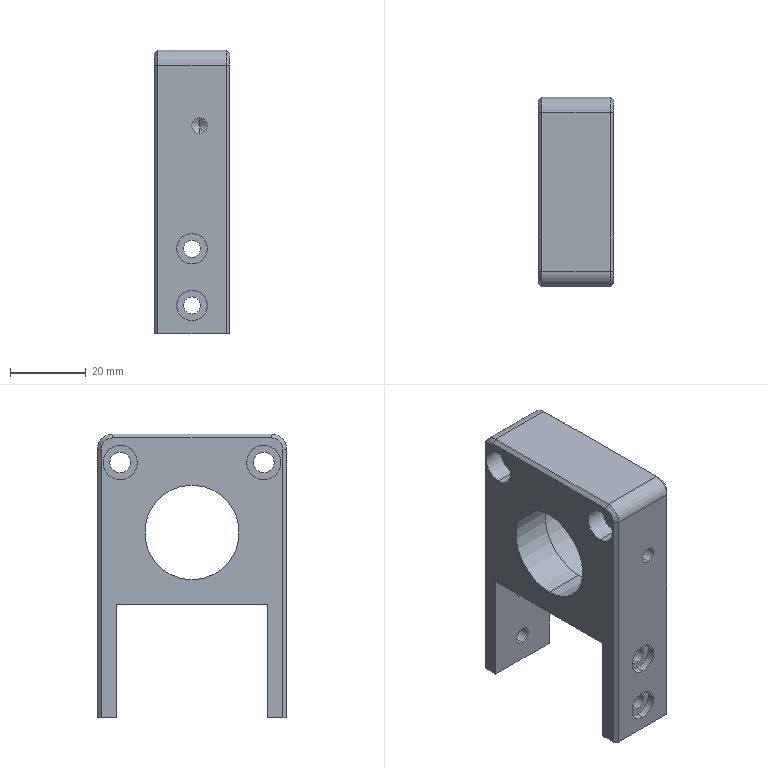Part | STEP file | PN_0002 | 1 solid | 65 faces | box 20 x 50 x 75 mm | volume 35811 mm3 | cylinder 34 | plane 23 | cone 8 | commonest cylinder face diameters 8 x10 4.5 x8 4.2 x4 5.5 x4 9 x4 25 x2